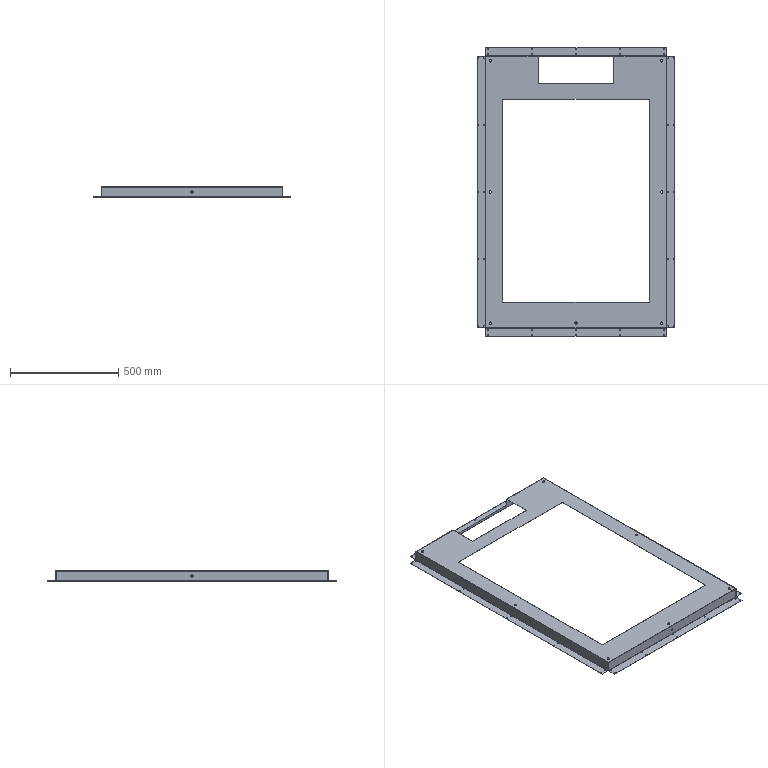Part | SolidWorks | features ICE 7, EdgeFlange 2, FlatPattern 1, SMBaseFlange 1, SheetMetal 1 | 1 solid | 184 faces | box 913 x 1333 x 48 mm | volume 715108 mm3 | cylinder 118 | plane 58 | spline 8 | commonest cylinder face diameters 4.2 x80 11 x14 0.4 x9 2.4 x9 10 x6